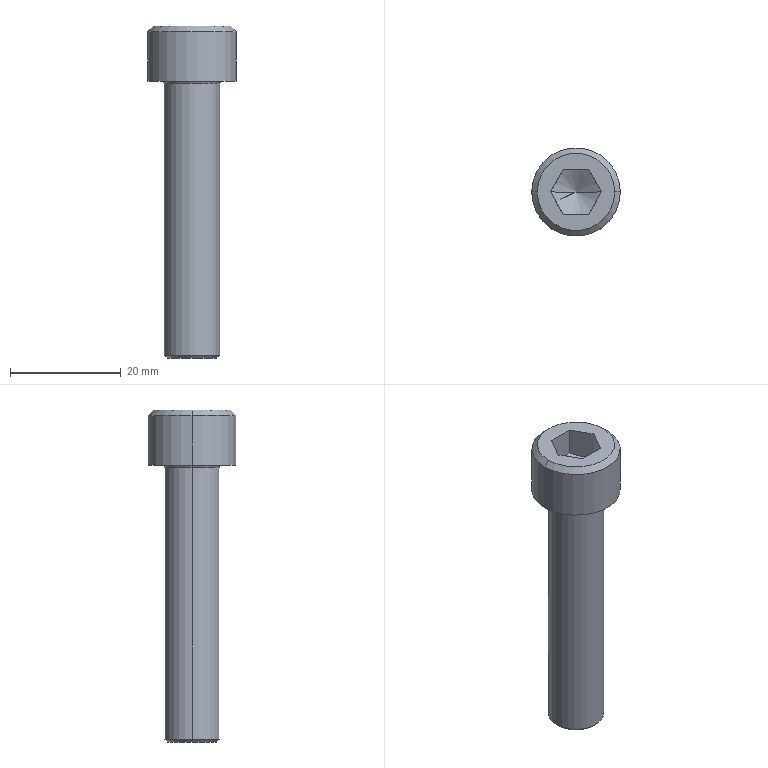Part | Creo | 1 solid | 23 faces | box 16 x 16 x 60 mm | volume 5576 mm3 | plane 9 | cone 6 | cylinder 4 | torus 4 | commonest cylinder face diameters 10 x2 16 x2
STEP:
#1=CARTESIAN_POINT('',(-126.381,37.995,-60.));
#2=VERTEX_POINT('',#1);
#3=CARTESIAN_POINT('',(-128.691,41.995,-60.));
#4=VERTEX_POINT('',#3);
#5=CARTESIAN_POINT('',(-126.381,37.995,-60.));
#6=CARTESIAN_POINT('',(-126.507,38.213,-60.073));
#7=CARTESIAN_POINT('',(-126.759,38.65,-60.201));
#8=CARTESIAN_POINT('',(-127.145,39.318,-60.327));
#9=CARTESIAN_POINT('',(-127.535,39.993,-60.372));
#10=CARTESIAN_POINT('',(-127.926,40.671,-60.328));
#11=CARTESIAN_POINT('',(-128.311,41.338,-60.201));
#12=CARTESIAN_POINT('',(-128.564,41.777,-60.073));
#13=CARTESIAN_POINT('',(-128.691,41.995,-60.));
#14=B_SPLINE_CURVE_WITH_KNOTS('',3,(#5,#6,#7,#8,#9,#10,#11,#12,#13),.UNSPECIFIED.,.F.,.F.,(4,1,1,1,1,1,4),(0.,0.1667,0.3333,0.5,0.6667,0.8333,1.),.UNSPECIFIED.);
#15=EDGE_CURVE('',#2,#4,#14,.T.);
#16=ORIENTED_EDGE('',*,*,#15,.F.);
#17=CARTESIAN_POINT('',(-131.,37.995,-62.667));
#18=VERTEX_POINT('',#17);
#19=CARTESIAN_POINT('',(-131.,37.995,-62.667));
#20=DIRECTION('',(0.866,0.,0.5));
#21=VECTOR('',#20,5.333);
#22=LINE('',#19,#21);
#23=EDGE_CURVE('',#18,#2,#22,.T.);
#24=ORIENTED_EDGE('',*,*,#23,.F.);
#25=CARTESIAN_POINT('',(-135.619,37.995,-60.));
#26=VERTEX_POINT('',#25);
#27=CARTESIAN_POINT('',(-131.,37.995,-62.667));
#28=DIRECTION('',(-0.866,0.,0.5));
#29=VECTOR('',#28,5.333);
#30=LINE('',#27,#29);
#31=EDGE_CURVE('',#18,#26,#30,.T.);
#32=ORIENTED_EDGE('',*,*,#31,.T.);
#33=CARTESIAN_POINT('',(-133.309,41.995,-60.));
#34=VERTEX_POINT('',#33);
#35=CARTESIAN_POINT('',(-133.309,41.995,-60.));
#36=CARTESIAN_POINT('',(-133.435,41.778,-60.073));
#37=CARTESIAN_POINT('',(-133.687,41.341,-60.201));
#38=CARTESIAN_POINT('',(-134.073,40.672,-60.327));
#39=CARTESIAN_POINT('',(-134.463,39.997,-60.372));
#40=CARTESIAN_POINT('',(-134.854,39.32,-60.328));
#41=CARTESIAN_POINT('',(-135.239,38.652,-60.201));
#42=CARTESIAN_POINT('',(-135.493,38.214,-60.073));
#43=CARTESIAN_POINT('',(-135.619,37.995,-60.));
#44=B_SPLINE_CURVE_WITH_KNOTS('',3,(#35,#36,#37,#38,#39,#40,#41,#42,#43),.UNSPECIFIED.,.F.,.F.,(4,1,1,1,1,1,4),(0.,0.1667,0.3333,0.5,0.6667,0.8333,1.),.UNSPECIFIED.);
#45=EDGE_CURVE('',#34,#26,#44,.T.);
#46=ORIENTED_EDGE('',*,*,#45,.F.);
#47=CARTESIAN_POINT('',(-128.691,41.995,-60.));
#48=CARTESIAN_POINT('',(-128.941,41.995,-60.072));
#49=CARTESIAN_POINT('',(-129.444,41.995,-60.2));
#50=CARTESIAN_POINT('',(-130.218,41.995,-60.327));
#51=CARTESIAN_POINT('',(-130.999,41.995,-60.372));
#52=CARTESIAN_POINT('',(-131.779,41.995,-60.328));
#53=CARTESIAN_POINT('',(-132.553,41.995,-60.201));
#54=CARTESIAN_POINT('',(-133.058,41.995,-60.073));
#55=CARTESIAN_POINT('',(-133.309,41.995,-60.));
#56=B_SPLINE_CURVE_WITH_KNOTS('',3,(#47,#48,#49,#50,#51,#52,#53,#54,#55),.UNSPECIFIED.,.F.,.F.,(4,1,1,1,1,1,4),(0.,0.1667,0.3333,0.5,0.6667,0.8333,1.),.UNSPECIFIED.);
#57=EDGE_CURVE('',#4,#34,#56,.T.);
#58=ORIENTED_EDGE('',*,*,#57,.F.);
#59=EDGE_LOOP('',(#16,#24,#32,#46,#58));
#60=FACE_OUTER_BOUND('',#59,.F.);
#61=CARTESIAN_POINT('',(-131.,37.995,-61.307));
#62=DIRECTION('',(0.,0.,1.));
#63=DIRECTION('',(1.,0.,0.));
#64=AXIS2_PLACEMENT_3D('',#61,#62,#63);
#65=CONICAL_SURFACE('',#64,2.356,60.);
#66=ADVANCED_FACE('',(#60),#65,.F.);
#67=CARTESIAN_POINT('',(-128.691,41.995,-55.));
#68=VERTEX_POINT('',#67);
#69=CARTESIAN_POINT('',(-126.381,37.995,-55.));
#70=VERTEX_POINT('',#69);
#71=CARTESIAN_POINT('',(-128.691,41.995,-55.));
#72=DIRECTION('',(0.5,-0.866,0.));
#73=VECTOR('',#72,4.619);
#74=LINE('',#71,#73);
#75=EDGE_CURVE('',#68,#70,#74,.T.);
#76=ORIENTED_EDGE('',*,*,#75,.T.);
#77=CARTESIAN_POINT('',(-126.381,37.995,-55.));
#78=DIRECTION('',(0.,0.,-1.));
#79=VECTOR('',#78,5.);
#80=LINE('',#77,#79);
#81=EDGE_CURVE('',#70,#2,#80,.T.);
#82=ORIENTED_EDGE('',*,*,#81,.T.);
#83=ORIENTED_EDGE('',*,*,#15,.T.);
#84=CARTESIAN_POINT('',(-128.691,41.995,-55.));
#85=DIRECTION('',(0.,0.,-1.));
#86=VECTOR('',#85,5.);
#87=LINE('',#84,#86);
#88=EDGE_CURVE('',#68,#4,#87,.T.);
#89=ORIENTED_EDGE('',*,*,#88,.F.);
#90=EDGE_LOOP('',(#76,#82,#83,#89));
#91=FACE_OUTER_BOUND('',#90,.F.);
#92=CARTESIAN_POINT('',(-128.691,41.995,-60.));
#93=DIRECTION('',(-0.866,-0.5,0.));
#94=DIRECTION('',(0.5,-0.866,0.));
#95=AXIS2_PLACEMENT_3D('',#92,#93,#94);
#96=PLANE('',#95);
#97=ADVANCED_FACE('',(#91),#96,.T.);
#98=CARTESIAN_POINT('',(-124.,37.995,-55.));
#99=VERTEX_POINT('',#98);
#100=CARTESIAN_POINT('',(-138.,37.995,-55.));
#101=VERTEX_POINT('',#100);
#102=CARTESIAN_POINT('',(-131.,37.995,-55.));
#103=DIRECTION('',(0.,0.,1.));
#104=DIRECTION('',(1.,0.,0.));
#105=AXIS2_PLACEMENT_3D('',#102,#103,#104);
#106=CIRCLE('',#105,7.);
#107=EDGE_CURVE('',#99,#101,#106,.T.);
#108=ORIENTED_EDGE('',*,*,#107,.F.);
#109=CARTESIAN_POINT('',(-131.,37.995,-55.));
#110=DIRECTION('',(0.,0.,1.));
#111=DIRECTION('',(-1.,0.,0.));
#112=AXIS2_PLACEMENT_3D('',#109,#110,#111);
#113=CIRCLE('',#112,7.);
#114=EDGE_CURVE('',#101,#99,#113,.T.);
#115=ORIENTED_EDGE('',*,*,#114,.F.);
#116=EDGE_LOOP('',(#108,#115));
#117=FACE_OUTER_BOUND('',#116,.F.);
#118=CARTESIAN_POINT('',(-128.691,33.995,-55.));
#119=VERTEX_POINT('',#118);
#120=CARTESIAN_POINT('',(-126.381,37.995,-55.));
#121=DIRECTION('',(-0.5,-0.866,0.));
#122=VECTOR('',#121,4.619);
#123=LINE('',#120,#122);
#124=EDGE_CURVE('',#70,#119,#123,.T.);
#125=ORIENTED_EDGE('',*,*,#124,.F.);
#126=ORIENTED_EDGE('',*,*,#75,.F.);
#127=CARTESIAN_POINT('',(-133.309,41.995,-55.));
#128=VERTEX_POINT('',#127);
#129=CARTESIAN_POINT('',(-128.691,41.995,-55.));
#130=DIRECTION('',(-1.,0.,0.));
#131=VECTOR('',#130,4.619);
#132=LINE('',#129,#131);
#133=EDGE_CURVE('',#68,#128,#132,.T.);
#134=ORIENTED_EDGE('',*,*,#133,.T.);
#135=CARTESIAN_POINT('',(-135.619,37.995,-55.));
#136=VERTEX_POINT('',#135);
#137=CARTESIAN_POINT('',(-135.619,37.995,-55.));
#138=DIRECTION('',(0.5,0.866,0.));
#139=VECTOR('',#138,4.619);
#140=LINE('',#137,#139);
#141=EDGE_CURVE('',#136,#128,#140,.T.);
#142=ORIENTED_EDGE('',*,*,#141,.F.);
#143=CARTESIAN_POINT('',(-133.309,33.995,-55.));
#144=VERTEX_POINT('',#143);
#145=CARTESIAN_POINT('',(-133.309,33.995,-55.));
#146=DIRECTION('',(-0.5,0.866,0.));
#147=VECTOR('',#146,4.619);
#148=LINE('',#145,#147);
#149=EDGE_CURVE('',#144,#136,#148,.T.);
#150=ORIENTED_EDGE('',*,*,#149,.F.);
#151=CARTESIAN_POINT('',(-133.309,33.995,-55.));
#152=DIRECTION('',(1.,0.,0.));
#153=VECTOR('',#152,4.619);
#154=LINE('',#151,#153);
#155=EDGE_CURVE('',#144,#119,#154,.T.);
#156=ORIENTED_EDGE('',*,*,#155,.T.);
#157=EDGE_LOOP('',(#125,#126,#134,#142,#150,#156));
#158=FACE_BOUND('',#157,.F.);
#159=CARTESIAN_POINT('',(-131.,37.995,-55.));
#160=DIRECTION('',(0.,0.,1.));
#161=DIRECTION('',(1.,0.,0.));
#162=AXIS2_PLACEMENT_3D('',#159,#160,#161);
#163=PLANE('',#162);
#164=ADVANCED_FACE('',(#117,#158),#163,.T.);
#165=CARTESIAN_POINT('',(-123.,37.995,-56.));
#166=VERTEX_POINT('',#165);
#167=CARTESIAN_POINT('',(-139.,37.995,-56.));
#168=VERTEX_POINT('',#167);
#169=CARTESIAN_POINT('',(-131.,37.995,-56.));
#170=DIRECTION('',(0.,0.,1.));
#171=DIRECTION('',(1.,0.,0.));
#172=AXIS2_PLACEMENT_3D('',#169,#170,#171);
#173=CIRCLE('',#172,8.);
#174=EDGE_CURVE('',#166,#168,#173,.T.);
#175=ORIENTED_EDGE('',*,*,#174,.F.);
#176=CARTESIAN_POINT('',(-124.,37.995,-55.));
#177=DIRECTION('',(0.7071,0.,-0.7071));
#178=VECTOR('',#177,1.414);
#179=LINE('',#176,#178);
#180=EDGE_CURVE('',#99,#166,#179,.T.);
#181=ORIENTED_EDGE('',*,*,#180,.F.);
#182=ORIENTED_EDGE('',*,*,#107,.T.);
#183=CARTESIAN_POINT('',(-138.,37.995,-55.));
#184=DIRECTION('',(-0.7071,0.,-0.7071));
#185=VECTOR('',#184,1.414);
#186=LINE('',#183,#185);
#187=EDGE_CURVE('',#101,#168,#186,.T.);
#188=ORIENTED_EDGE('',*,*,#187,.T.);
#189=EDGE_LOOP('',(#175,#181,#182,#188));
#190=FACE_OUTER_BOUND('',#189,.F.);
#191=CARTESIAN_POINT('',(-131.,37.995,-55.5));
#192=DIRECTION('',(0.,0.,-1.));
#193=DIRECTION('',(-1.,0.,0.));
#194=AXIS2_PLACEMENT_3D('',#191,#192,#193);
#195=CONICAL_SURFACE('',#194,7.5,45.);
#196=ADVANCED_FACE('',(#190),#195,.T.);
#197=ORIENTED_EDGE('',*,*,#174,.T.);
#198=CARTESIAN_POINT('',(-139.,37.995,-65.));
#199=VERTEX_POINT('',#198);
#200=CARTESIAN_POINT('',(-139.,37.995,-65.));
#201=DIRECTION('',(0.,0.,1.));
#202=VECTOR('',#201,9.);
#203=LINE('',#200,#202);
#204=EDGE_CURVE('',#199,#168,#203,.T.);
#205=ORIENTED_EDGE('',*,*,#204,.F.);
#206=CARTESIAN_POINT('',(-123.,37.995,-65.));
#207=VERTEX_POINT('',#206);
#208=CARTESIAN_POINT('',(-131.,37.995,-65.));
#209=DIRECTION('',(0.,0.,-1.));
#210=DIRECTION('',(-1.,0.,0.));
#211=AXIS2_PLACEMENT_3D('',#208,#209,#210);
#212=CIRCLE('',#211,8.);
#213=EDGE_CURVE('',#199,#207,#212,.T.);
#214=ORIENTED_EDGE('',*,*,#213,.T.);
#215=CARTESIAN_POINT('',(-123.,37.995,-65.));
#216=DIRECTION('',(0.,0.,1.));
#217=VECTOR('',#216,9.);
#218=LINE('',#215,#217);
#219=EDGE_CURVE('',#207,#166,#218,.T.);
#220=ORIENTED_EDGE('',*,*,#219,.T.);
#221=EDGE_LOOP('',(#197,#205,#214,#220));
#222=FACE_OUTER_BOUND('',#221,.F.);
#223=CARTESIAN_POINT('',(-131.,37.995,-65.));
#224=DIRECTION('',(0.,0.,1.));
#225=DIRECTION('',(1.,0.,0.));
#226=AXIS2_PLACEMENT_3D('',#223,#224,#225);
#227=CYLINDRICAL_SURFACE('',#226,8.);
#228=ADVANCED_FACE('',(#222),#227,.T.);
#229=CARTESIAN_POINT('',(-131.,37.995,-56.));
#230=DIRECTION('',(0.,0.,1.));
#231=DIRECTION('',(-1.,0.,0.));
#232=AXIS2_PLACEMENT_3D('',#229,#230,#231);
#233=CIRCLE('',#232,8.);
#234=EDGE_CURVE('',#168,#166,#233,.T.);
#235=ORIENTED_EDGE('',*,*,#234,.T.);
#236=ORIENTED_EDGE('',*,*,#219,.F.);
#237=CARTESIAN_POINT('',(-131.,37.995,-65.));
#238=DIRECTION('',(0.,0.,-1.));
#239=DIRECTION('',(1.,0.,0.));
#240=AXIS2_PLACEMENT_3D('',#237,#238,#239);
#241=CIRCLE('',#240,8.);
#242=EDGE_CURVE('',#207,#199,#241,.T.);
#243=ORIENTED_EDGE('',*,*,#242,.T.);
#244=ORIENTED_EDGE('',*,*,#204,.T.);
#245=EDGE_LOOP('',(#235,#236,#243,#244));
#246=FACE_OUTER_BOUND('',#245,.F.);
#247=CARTESIAN_POINT('',(-131.,37.995,-65.));
#248=DIRECTION('',(0.,0.,1.));
#249=DIRECTION('',(1.,0.,0.));
#250=AXIS2_PLACEMENT_3D('',#247,#248,#249);
#251=CYLINDRICAL_SURFACE('',#250,8.);
#252=ADVANCED_FACE('',(#246),#251,.T.);
#253=ORIENTED_EDGE('',*,*,#234,.F.);
#254=ORIENTED_EDGE('',*,*,#187,.F.);
#255=ORIENTED_EDGE('',*,*,#114,.T.);
#256=ORIENTED_EDGE('',*,*,#180,.T.);
#257=EDGE_LOOP('',(#253,#254,#255,#256));
#258=FACE_OUTER_BOUND('',#257,.F.);
#259=CARTESIAN_POINT('',(-131.,37.995,-55.5));
#260=DIRECTION('',(0.,0.,-1.));
#261=DIRECTION('',(-1.,0.,0.));
#262=AXIS2_PLACEMENT_3D('',#259,#260,#261);
#263=CONICAL_SURFACE('',#262,7.5,45.);
#264=ADVANCED_FACE('',(#258),#263,.T.);
#265=ORIENTED_EDGE('',*,*,#242,.F.);
#266=ORIENTED_EDGE('',*,*,#213,.F.);
#267=EDGE_LOOP('',(#265,#266));
#268=FACE_OUTER_BOUND('',#267,.F.);
#269=CARTESIAN_POINT('',(-125.6,37.995,-65.));
#270=VERTEX_POINT('',#269);
#271=CARTESIAN_POINT('',(-136.4,37.995,-65.));
#272=VERTEX_POINT('',#271);
#273=CARTESIAN_POINT('',(-131.,37.995,-65.));
#274=DIRECTION('',(0.,0.,1.));
#275=DIRECTION('',(1.,0.,0.));
#276=AXIS2_PLACEMENT_3D('',#273,#274,#275);
#277=CIRCLE('',#276,5.4);
#278=EDGE_CURVE('',#270,#272,#277,.T.);
#279=ORIENTED_EDGE('',*,*,#278,.F.);
#280=CARTESIAN_POINT('',(-131.,37.995,-65.));
#281=DIRECTION('',(0.,0.,1.));
#282=DIRECTION('',(-1.,0.,0.));
#283=AXIS2_PLACEMENT_3D('',#280,#281,#282);
#284=CIRCLE('',#283,5.4);
#285=EDGE_CURVE('',#272,#270,#284,.T.);
#286=ORIENTED_EDGE('',*,*,#285,.F.);
#287=EDGE_LOOP('',(#279,#286));
#288=FACE_BOUND('',#287,.F.);
#289=CARTESIAN_POINT('',(-131.,37.995,-65.));
#290=DIRECTION('',(0.,0.,1.));
#291=DIRECTION('',(1.,0.,0.));
#292=AXIS2_PLACEMENT_3D('',#289,#290,#291);
#293=PLANE('',#292);
#294=ADVANCED_FACE('',(#268,#288),#293,.F.);
#295=ORIENTED_EDGE('',*,*,#278,.T.);
#296=CARTESIAN_POINT('',(-136.117,37.995,-65.117));
#297=VERTEX_POINT('',#296);
#298=CARTESIAN_POINT('',(-136.4,37.995,-65.4));
#299=DIRECTION('',(0.,1.,0.));
#300=DIRECTION('',(0.,0.,1.));
#301=AXIS2_PLACEMENT_3D('',#298,#299,#300);
#302=CIRCLE('',#301,0.4);
#303=EDGE_CURVE('',#272,#297,#302,.T.);
#304=ORIENTED_EDGE('',*,*,#303,.T.);
#305=CARTESIAN_POINT('',(-125.883,37.995,-65.117));
#306=VERTEX_POINT('',#305);
#307=CARTESIAN_POINT('',(-131.,37.995,-65.117));
#308=DIRECTION('',(0.,0.,1.));
#309=DIRECTION('',(1.,0.,0.));
#310=AXIS2_PLACEMENT_3D('',#307,#308,#309);
#311=CIRCLE('',#310,5.117);
#312=EDGE_CURVE('',#306,#297,#311,.T.);
#313=ORIENTED_EDGE('',*,*,#312,.F.);
#314=CARTESIAN_POINT('',(-125.6,37.995,-65.4));
#315=DIRECTION('',(0.,-1.,0.));
#316=DIRECTION('',(0.,0.,1.));
#317=AXIS2_PLACEMENT_3D('',#314,#315,#316);
#318=CIRCLE('',#317,0.4);
#319=EDGE_CURVE('',#270,#306,#318,.T.);
#320=ORIENTED_EDGE('',*,*,#319,.F.);
#321=EDGE_LOOP('',(#295,#304,#313,#320));
#322=FACE_OUTER_BOUND('',#321,.F.);
#323=CARTESIAN_POINT('',(-131.,37.995,-65.4));
#324=DIRECTION('',(0.,0.,1.));
#325=DIRECTION('',(1.,0.,0.));
#326=AXIS2_PLACEMENT_3D('',#323,#324,#325);
#327=TOROIDAL_SURFACE('',#326,5.4,0.4);
#328=ADVANCED_FACE('',(#322),#327,.F.);
#329=ORIENTED_EDGE('',*,*,#285,.T.);
#330=ORIENTED_EDGE('',*,*,#319,.T.);
#331=CARTESIAN_POINT('',(-131.,37.995,-65.117));
#332=DIRECTION('',(0.,0.,1.));
#333=DIRECTION('',(-1.,0.,0.));
#334=AXIS2_PLACEMENT_3D('',#331,#332,#333);
#335=CIRCLE('',#334,5.117);
#336=EDGE_CURVE('',#297,#306,#335,.T.);
#337=ORIENTED_EDGE('',*,*,#336,.F.);
#338=ORIENTED_EDGE('',*,*,#303,.F.);
#339=EDGE_LOOP('',(#329,#330,#337,#338));
#340=FACE_OUTER_BOUND('',#339,.F.);
#341=CARTESIAN_POINT('',(-131.,37.995,-65.4));
#342=DIRECTION('',(0.,0.,1.));
#343=DIRECTION('',(1.,0.,0.));
#344=AXIS2_PLACEMENT_3D('',#341,#342,#343);
#345=TOROIDAL_SURFACE('',#344,5.4,0.4);
#346=ADVANCED_FACE('',(#340),#345,.F.);
#347=CARTESIAN_POINT('',(-136.,37.995,-65.4));
#348=VERTEX_POINT('',#347);
#349=CARTESIAN_POINT('',(-126.,37.995,-65.4));
#350=VERTEX_POINT('',#349);
#351=CARTESIAN_POINT('',(-131.,37.995,-65.4));
#352=DIRECTION('',(0.,0.,1.));
#353=DIRECTION('',(-1.,0.,0.));
#354=AXIS2_PLACEMENT_3D('',#351,#352,#353);
#355=CIRCLE('',#354,5.);
#356=EDGE_CURVE('',#348,#350,#355,.T.);
#357=ORIENTED_EDGE('',*,*,#356,.F.);
#358=CARTESIAN_POINT('',(-136.4,37.995,-65.4));
#359=DIRECTION('',(0.,1.,0.));
#360=DIRECTION('',(0.7071,0.,0.7071));
#361=AXIS2_PLACEMENT_3D('',#358,#359,#360);
#362=CIRCLE('',#361,0.4);
#363=EDGE_CURVE('',#297,#348,#362,.T.);
#364=ORIENTED_EDGE('',*,*,#363,.F.);
#365=ORIENTED_EDGE('',*,*,#336,.T.);
#366=CARTESIAN_POINT('',(-125.6,37.995,-65.4));
#367=DIRECTION('',(0.,-1.,0.));
#368=DIRECTION('',(-0.7071,0.,0.7071));
#369=AXIS2_PLACEMENT_3D('',#366,#367,#368);
#370=CIRCLE('',#369,0.4);
#371=EDGE_CURVE('',#306,#350,#370,.T.);
#372=ORIENTED_EDGE('',*,*,#371,.T.);
#373=EDGE_LOOP('',(#357,#364,#365,#372));
#374=FACE_OUTER_BOUND('',#373,.F.);
#375=CARTESIAN_POINT('',(-131.,37.995,-65.4));
#376=DIRECTION('',(0.,0.,1.));
#377=DIRECTION('',(1.,0.,0.));
#378=AXIS2_PLACEMENT_3D('',#375,#376,#377);
#379=TOROIDAL_SURFACE('',#378,5.4,0.4);
#380=ADVANCED_FACE('',(#374),#379,.F.);
#381=CARTESIAN_POINT('',(-126.,37.995,-114.5));
#382=VERTEX_POINT('',#381);
#383=CARTESIAN_POINT('',(-136.,37.995,-114.5));
#384=VERTEX_POINT('',#383);
#385=CARTESIAN_POINT('',(-131.,37.995,-114.5));
#386=DIRECTION('',(0.,0.,-1.));
#387=DIRECTION('',(1.,0.,0.));
#388=AXIS2_PLACEMENT_3D('',#385,#386,#387);
#389=CIRCLE('',#388,5.);
#390=EDGE_CURVE('',#382,#384,#389,.T.);
#391=ORIENTED_EDGE('',*,*,#390,.T.);
#392=CARTESIAN_POINT('',(-136.,37.995,-114.5));
#393=DIRECTION('',(0.,0.,1.));
#394=VECTOR('',#393,49.1);
#395=LINE('',#392,#394);
#396=EDGE_CURVE('',#384,#348,#395,.T.);
#397=ORIENTED_EDGE('',*,*,#396,.T.);
#398=ORIENTED_EDGE('',*,*,#356,.T.);
#399=CARTESIAN_POINT('',(-126.,37.995,-114.5));
#400=DIRECTION('',(0.,0.,1.));
#401=VECTOR('',#400,49.1);
#402=LINE('',#399,#401);
#403=EDGE_CURVE('',#382,#350,#402,.T.);
#404=ORIENTED_EDGE('',*,*,#403,.F.);
#405=EDGE_LOOP('',(#391,#397,#398,#404));
#406=FACE_OUTER_BOUND('',#405,.F.);
#407=CARTESIAN_POINT('',(-131.,37.995,-115.));
#408=DIRECTION('',(0.,0.,1.));
#409=DIRECTION('',(1.,0.,0.));
#410=AXIS2_PLACEMENT_3D('',#407,#408,#409);
#411=CYLINDRICAL_SURFACE('',#410,5.);
#412=ADVANCED_FACE('',(#406),#411,.T.);
#413=CARTESIAN_POINT('',(-126.5,37.995,-115.));
#414=VERTEX_POINT('',#413);
#415=CARTESIAN_POINT('',(-135.5,37.995,-115.));
#416=VERTEX_POINT('',#415);
#417=CARTESIAN_POINT('',(-131.,37.995,-115.));
#418=DIRECTION('',(0.,0.,-1.));
#419=DIRECTION('',(1.,0.,0.));
#420=AXIS2_PLACEMENT_3D('',#417,#418,#419);
#421=CIRCLE('',#420,4.5);
#422=EDGE_CURVE('',#414,#416,#421,.T.);
#423=ORIENTED_EDGE('',*,*,#422,.T.);
#424=CARTESIAN_POINT('',(-135.5,37.995,-115.));
#425=DIRECTION('',(-0.7071,0.,0.7071));
#426=VECTOR('',#425,0.7071);
#427=LINE('',#424,#426);
#428=EDGE_CURVE('',#416,#384,#427,.T.);
#429=ORIENTED_EDGE('',*,*,#428,.T.);
#430=ORIENTED_EDGE('',*,*,#390,.F.);
#431=CARTESIAN_POINT('',(-126.5,37.995,-115.));
#432=DIRECTION('',(0.7071,0.,0.7071));
#433=VECTOR('',#432,0.7071);
#434=LINE('',#431,#433);
#435=EDGE_CURVE('',#414,#382,#434,.T.);
#436=ORIENTED_EDGE('',*,*,#435,.F.);
#437=EDGE_LOOP('',(#423,#429,#430,#436));
#438=FACE_OUTER_BOUND('',#437,.F.);
#439=CARTESIAN_POINT('',(-131.,37.995,-114.75));
#440=DIRECTION('',(0.,0.,1.));
#441=DIRECTION('',(1.,0.,0.));
#442=AXIS2_PLACEMENT_3D('',#439,#440,#441);
#443=CONICAL_SURFACE('',#442,4.75,45.);
#444=ADVANCED_FACE('',(#438),#443,.T.);
#445=ORIENTED_EDGE('',*,*,#422,.F.);
#446=CARTESIAN_POINT('',(-131.,37.995,-115.));
#447=DIRECTION('',(0.,0.,-1.));
#448=DIRECTION('',(-1.,0.,0.));
#449=AXIS2_PLACEMENT_3D('',#446,#447,#448);
#450=CIRCLE('',#449,4.5);
#451=EDGE_CURVE('',#416,#414,#450,.T.);
#452=ORIENTED_EDGE('',*,*,#451,.F.);
#453=EDGE_LOOP('',(#445,#452));
#454=FACE_OUTER_BOUND('',#453,.F.);
#455=CARTESIAN_POINT('',(-131.,37.995,-115.));
#456=DIRECTION('',(0.,0.,1.));
#457=DIRECTION('',(1.,0.,0.));
#458=AXIS2_PLACEMENT_3D('',#455,#456,#457);
#459=PLANE('',#458);
#460=ADVANCED_FACE('',(#454),#459,.F.);
#461=ORIENTED_EDGE('',*,*,#451,.T.);
#462=ORIENTED_EDGE('',*,*,#435,.T.);
#463=CARTESIAN_POINT('',(-131.,37.995,-114.5));
#464=DIRECTION('',(0.,0.,-1.));
#465=DIRECTION('',(-1.,0.,0.));
#466=AXIS2_PLACEMENT_3D('',#463,#464,#465);
#467=CIRCLE('',#466,5.);
#468=EDGE_CURVE('',#384,#382,#467,.T.);
#469=ORIENTED_EDGE('',*,*,#468,.F.);
#470=ORIENTED_EDGE('',*,*,#428,.F.);
#471=EDGE_LOOP('',(#461,#462,#469,#470));
#472=FACE_OUTER_BOUND('',#471,.F.);
#473=CARTESIAN_POINT('',(-131.,37.995,-114.75));
#474=DIRECTION('',(0.,0.,1.));
#475=DIRECTION('',(1.,0.,0.));
#476=AXIS2_PLACEMENT_3D('',#473,#474,#475);
#477=CONICAL_SURFACE('',#476,4.75,45.);
#478=ADVANCED_FACE('',(#472),#477,.T.);
#479=ORIENTED_EDGE('',*,*,#468,.T.);
#480=ORIENTED_EDGE('',*,*,#403,.T.);
#481=CARTESIAN_POINT('',(-131.,37.995,-65.4));
#482=DIRECTION('',(0.,0.,1.));
#483=DIRECTION('',(1.,0.,0.));
#484=AXIS2_PLACEMENT_3D('',#481,#482,#483);
#485=CIRCLE('',#484,5.);
#486=EDGE_CURVE('',#350,#348,#485,.T.);
#487=ORIENTED_EDGE('',*,*,#486,.T.);
#488=ORIENTED_EDGE('',*,*,#396,.F.);
#489=EDGE_LOOP('',(#479,#480,#487,#488));
#490=FACE_OUTER_BOUND('',#489,.F.);
#491=CARTESIAN_POINT('',(-131.,37.995,-115.));
#492=DIRECTION('',(0.,0.,1.));
#493=DIRECTION('',(1.,0.,0.));
#494=AXIS2_PLACEMENT_3D('',#491,#492,#493);
#495=CYLINDRICAL_SURFACE('',#494,5.);
#496=ADVANCED_FACE('',(#490),#495,.T.);
#497=ORIENTED_EDGE('',*,*,#486,.F.);
#498=ORIENTED_EDGE('',*,*,#371,.F.);
#499=ORIENTED_EDGE('',*,*,#312,.T.);
#500=ORIENTED_EDGE('',*,*,#363,.T.);
#501=EDGE_LOOP('',(#497,#498,#499,#500));
#502=FACE_OUTER_BOUND('',#501,.F.);
#503=CARTESIAN_POINT('',(-131.,37.995,-65.4));
#504=DIRECTION('',(0.,0.,1.));
#505=DIRECTION('',(1.,0.,0.));
#506=AXIS2_PLACEMENT_3D('',#503,#504,#505);
#507=TOROIDAL_SURFACE('',#506,5.4,0.4);
#508=ADVANCED_FACE('',(#502),#507,.F.);
#509=ORIENTED_EDGE('',*,*,#124,.T.);
#510=CARTESIAN_POINT('',(-128.691,33.995,-60.));
#511=VERTEX_POINT('',#510);
#512=CARTESIAN_POINT('',(-128.691,33.995,-55.));
#513=DIRECTION('',(0.,0.,-1.));
#514=VECTOR('',#513,5.);
#515=LINE('',#512,#514);
#516=EDGE_CURVE('',#119,#511,#515,.T.);
#517=ORIENTED_EDGE('',*,*,#516,.T.);
#518=CARTESIAN_POINT('',(-128.691,33.995,-60.));
#519=CARTESIAN_POINT('',(-128.565,34.213,-60.073));
#520=CARTESIAN_POINT('',(-128.313,34.65,-60.201));
#521=CARTESIAN_POINT('',(-127.927,35.318,-60.327));
#522=CARTESIAN_POINT('',(-127.537,35.993,-60.372));
#523=CARTESIAN_POINT('',(-127.146,36.671,-60.328));
#524=CARTESIAN_POINT('',(-126.761,37.338,-60.201));
#525=CARTESIAN_POINT('',(-126.507,37.777,-60.073));
#526=CARTESIAN_POINT('',(-126.381,37.995,-60.));
#527=B_SPLINE_CURVE_WITH_KNOTS('',3,(#518,#519,#520,#521,#522,#523,#524,#525,#526),.UNSPECIFIED.,.F.,.F.,(4,1,1,1,1,1,4),(0.,0.1667,0.3333,0.5,0.6667,0.8333,1.),.UNSPECIFIED.);
#528=EDGE_CURVE('',#511,#2,#527,.T.);
#529=ORIENTED_EDGE('',*,*,#528,.T.);
#530=ORIENTED_EDGE('',*,*,#81,.F.);
#531=EDGE_LOOP('',(#509,#517,#529,#530));
#532=FACE_OUTER_BOUND('',#531,.F.);
#533=CARTESIAN_POINT('',(-126.381,37.995,-60.));
#534=DIRECTION('',(-0.866,0.5,0.));
#535=DIRECTION('',(-0.5,-0.866,0.));
#536=AXIS2_PLACEMENT_3D('',#533,#534,#535);
#537=PLANE('',#536);
#538=ADVANCED_FACE('',(#532),#537,.T.);
#539=ORIENTED_EDGE('',*,*,#155,.F.);
#540=CARTESIAN_POINT('',(-133.309,33.995,-60.));
#541=VERTEX_POINT('',#540);
#542=CARTESIAN_POINT('',(-133.309,33.995,-55.));
#543=DIRECTION('',(0.,0.,-1.));
#544=VECTOR('',#543,5.);
#545=LINE('',#542,#544);
#546=EDGE_CURVE('',#144,#541,#545,.T.);
#547=ORIENTED_EDGE('',*,*,#546,.T.);
#548=CARTESIAN_POINT('',(-133.309,33.995,-60.));
#549=CARTESIAN_POINT('',(-133.058,33.995,-60.073));
#550=CARTESIAN_POINT('',(-132.553,33.995,-60.201));
#551=CARTESIAN_POINT('',(-131.779,33.995,-60.328));
#552=CARTESIAN_POINT('',(-130.999,33.995,-60.372));
#553=CARTESIAN_POINT('',(-130.218,33.995,-60.327));
#554=CARTESIAN_POINT('',(-129.444,33.995,-60.2));
#555=CARTESIAN_POINT('',(-128.941,33.995,-60.072));
#556=CARTESIAN_POINT('',(-128.691,33.995,-60.));
#557=B_SPLINE_CURVE_WITH_KNOTS('',3,(#548,#549,#550,#551,#552,#553,#554,#555,#556),.UNSPECIFIED.,.F.,.F.,(4,1,1,1,1,1,4),(0.,0.1667,0.3333,0.5,0.6667,0.8333,1.),.UNSPECIFIED.);
#558=EDGE_CURVE('',#541,#511,#557,.T.);
#559=ORIENTED_EDGE('',*,*,#558,.T.);
#560=ORIENTED_EDGE('',*,*,#516,.F.);
#561=EDGE_LOOP('',(#539,#547,#559,#560));
#562=FACE_OUTER_BOUND('',#561,.F.);
#563=CARTESIAN_POINT('',(-128.691,33.995,-60.));
#564=DIRECTION('',(0.,1.,0.));
#565=DIRECTION('',(0.,0.,1.));
#566=AXIS2_PLACEMENT_3D('',#563,#564,#565);
#567=PLANE('',#566);
#568=ADVANCED_FACE('',(#562),#567,.T.);
#569=ORIENTED_EDGE('',*,*,#149,.T.);
#570=CARTESIAN_POINT('',(-135.619,37.995,-55.));
#571=DIRECTION('',(0.,0.,-1.));
#572=VECTOR('',#571,5.);
#573=LINE('',#570,#572);
#574=EDGE_CURVE('',#136,#26,#573,.T.);
#575=ORIENTED_EDGE('',*,*,#574,.T.);
#576=CARTESIAN_POINT('',(-135.619,37.995,-60.));
#577=CARTESIAN_POINT('',(-135.493,37.777,-60.073));
#578=CARTESIAN_POINT('',(-135.239,37.338,-60.201));
#579=CARTESIAN_POINT('',(-134.854,36.671,-60.328));
#580=CARTESIAN_POINT('',(-134.463,35.993,-60.372));
#581=CARTESIAN_POINT('',(-134.073,35.318,-60.327));
#582=CARTESIAN_POINT('',(-133.687,34.65,-60.201));
#583=CARTESIAN_POINT('',(-133.435,34.213,-60.073));
#584=CARTESIAN_POINT('',(-133.309,33.995,-60.));
#585=B_SPLINE_CURVE_WITH_KNOTS('',3,(#576,#577,#578,#579,#580,#581,#582,#583,#584),.UNSPECIFIED.,.F.,.F.,(4,1,1,1,1,1,4),(0.,0.1667,0.3333,0.5,0.6667,0.8333,1.),.UNSPECIFIED.);
#586=EDGE_CURVE('',#26,#541,#585,.T.);
#587=ORIENTED_EDGE('',*,*,#586,.T.);
#588=ORIENTED_EDGE('',*,*,#546,.F.);
#589=EDGE_LOOP('',(#569,#575,#587,#588));
#590=FACE_OUTER_BOUND('',#589,.F.);
#591=CARTESIAN_POINT('',(-133.309,33.995,-60.));
#592=DIRECTION('',(0.866,0.5,0.));
#593=DIRECTION('',(-0.5,0.866,0.));
#594=AXIS2_PLACEMENT_3D('',#591,#592,#593);
#595=PLANE('',#594);
#596=ADVANCED_FACE('',(#590),#595,.T.);
#597=ORIENTED_EDGE('',*,*,#141,.T.);
#598=CARTESIAN_POINT('',(-133.309,41.995,-55.));
#599=DIRECTION('',(0.,0.,-1.));
#600=VECTOR('',#599,5.);
#601=LINE('',#598,#600);
#602=EDGE_CURVE('',#128,#34,#601,.T.);
#603=ORIENTED_EDGE('',*,*,#602,.T.);
#604=ORIENTED_EDGE('',*,*,#45,.T.);
#605=ORIENTED_EDGE('',*,*,#574,.F.);
#606=EDGE_LOOP('',(#597,#603,#604,#605));
#607=FACE_OUTER_BOUND('',#606,.F.);
#608=CARTESIAN_POINT('',(-135.619,37.995,-60.));
#609=DIRECTION('',(0.866,-0.5,0.));
#610=DIRECTION('',(0.5,0.866,0.));
#611=AXIS2_PLACEMENT_3D('',#608,#609,#610);
#612=PLANE('',#611);
#613=ADVANCED_FACE('',(#607),#612,.T.);
#614=ORIENTED_EDGE('',*,*,#133,.F.);
#615=ORIENTED_EDGE('',*,*,#88,.T.);
#616=ORIENTED_EDGE('',*,*,#57,.T.);
#617=ORIENTED_EDGE('',*,*,#602,.F.);
#618=EDGE_LOOP('',(#614,#615,#616,#617));
#619=FACE_OUTER_BOUND('',#618,.F.);
#620=CARTESIAN_POINT('',(-133.309,41.995,-60.));
#621=DIRECTION('',(0.,-1.,0.));
#622=DIRECTION('',(0.,0.,-1.));
#623=AXIS2_PLACEMENT_3D('',#620,#621,#622);
#624=PLANE('',#623);
#625=ADVANCED_FACE('',(#619),#624,.T.);
#626=ORIENTED_EDGE('',*,*,#586,.F.);
#627=ORIENTED_EDGE('',*,*,#31,.F.);
#628=ORIENTED_EDGE('',*,*,#23,.T.);
#629=ORIENTED_EDGE('',*,*,#528,.F.);
#630=ORIENTED_EDGE('',*,*,#558,.F.);
#631=EDGE_LOOP('',(#626,#627,#628,#629,#630));
#632=FACE_OUTER_BOUND('',#631,.F.);
#633=CARTESIAN_POINT('',(-131.,37.995,-61.307));
#634=DIRECTION('',(0.,0.,1.));
#635=DIRECTION('',(1.,0.,0.));
#636=AXIS2_PLACEMENT_3D('',#633,#634,#635);
#637=CONICAL_SURFACE('',#636,2.356,60.);
#638=ADVANCED_FACE('',(#632),#637,.F.);
#639=CLOSED_SHELL('',(#66,#97,#164,#196,#228,#252,#264,#294,#328,#346,#380,#412,#444,#460,#478,#496,#508,#538,#568,#596,#613,#625,#638));
#640=MANIFOLD_SOLID_BREP('',#639);
#641=(LENGTH_UNIT()NAMED_UNIT(*)SI_UNIT(.MILLI.,.METRE.));
#642=UNCERTAINTY_MEASURE_WITH_UNIT(LENGTH_MEASURE(0.006412),#641,'','');
#643=(NAMED_UNIT(*)PLANE_ANGLE_UNIT()SI_UNIT($,.RADIAN.));
#644=PLANE_ANGLE_MEASURE_WITH_UNIT(PLANE_ANGLE_MEASURE(0.01745),#643);
#645=(CONVERSION_BASED_UNIT('DEGREE',#644)NAMED_UNIT(*)PLANE_ANGLE_UNIT());
#646=(NAMED_UNIT(*)SI_UNIT($,.STERADIAN.)SOLID_ANGLE_UNIT());
#647=(GEOMETRIC_REPRESENTATION_CONTEXT(3)GLOBAL_UNCERTAINTY_ASSIGNED_CONTEXT((#642))GLOBAL_UNIT_ASSIGNED_CONTEXT((#641,#645,#646))REPRESENTATION_CONTEXT('',''));
#648=ADVANCED_BREP_SHAPE_REPRESENTATION('',(#640),#647);